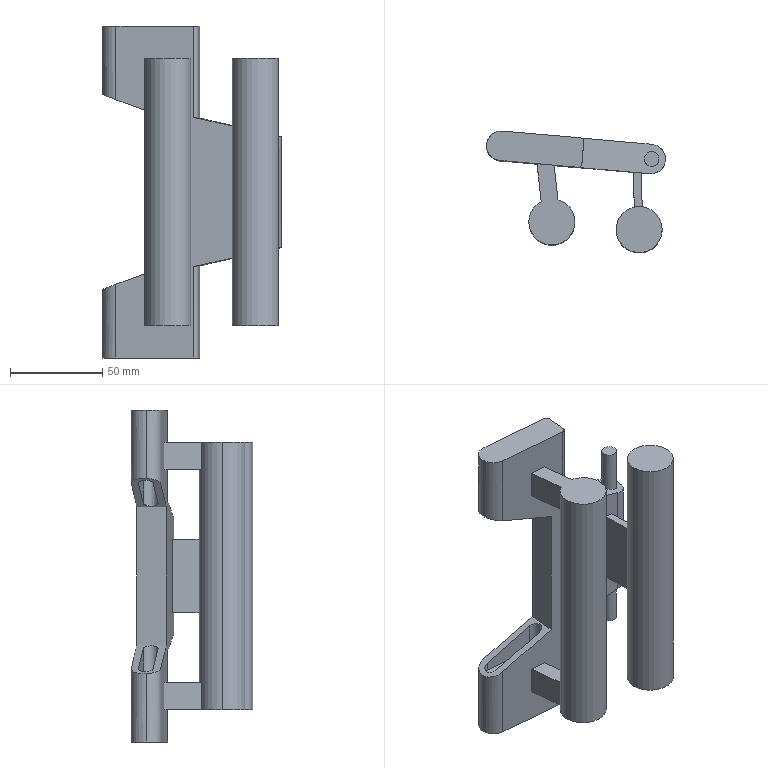Part | SolidWorks | features ICE 6, RefPoint 4, Fillet 2, Extrusion 1, MirrorPattern 1 | 1 solid | 57 faces | box 97.078 x 65.941 x 180 mm | volume 283713 mm3 | plane 33 | cylinder 24 | commonest cylinder face diameters 8 x10 16 x6 4 x4 25 x4